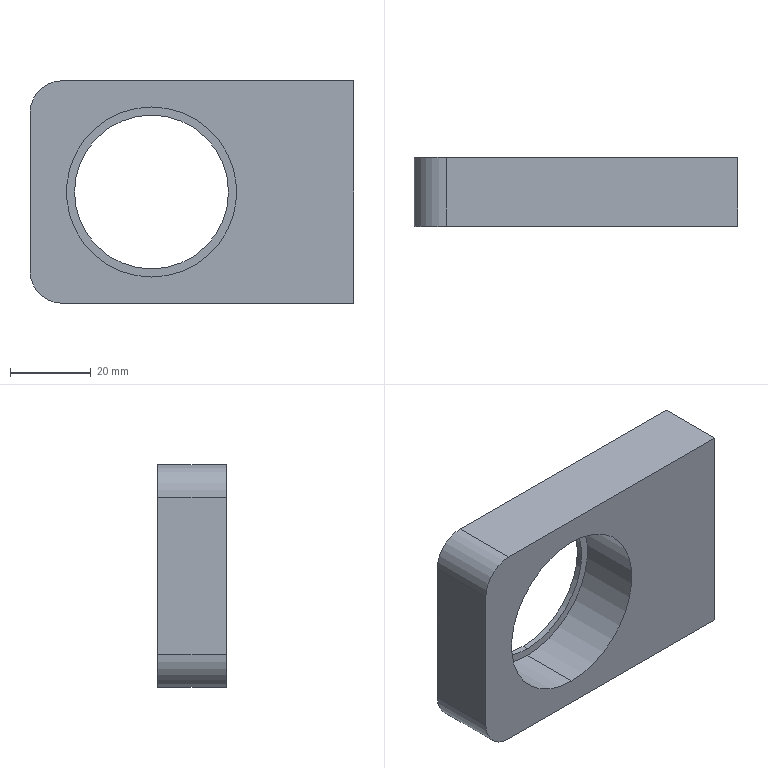Part | STEP file | 1 solid | 25 faces | box 80 x 17 x 55 mm | volume 50244 mm3 | cylinder 12 | plane 7 | cone 6 | commonest cylinder face diameters 5 x6 16 x2 38 x2 42 x2